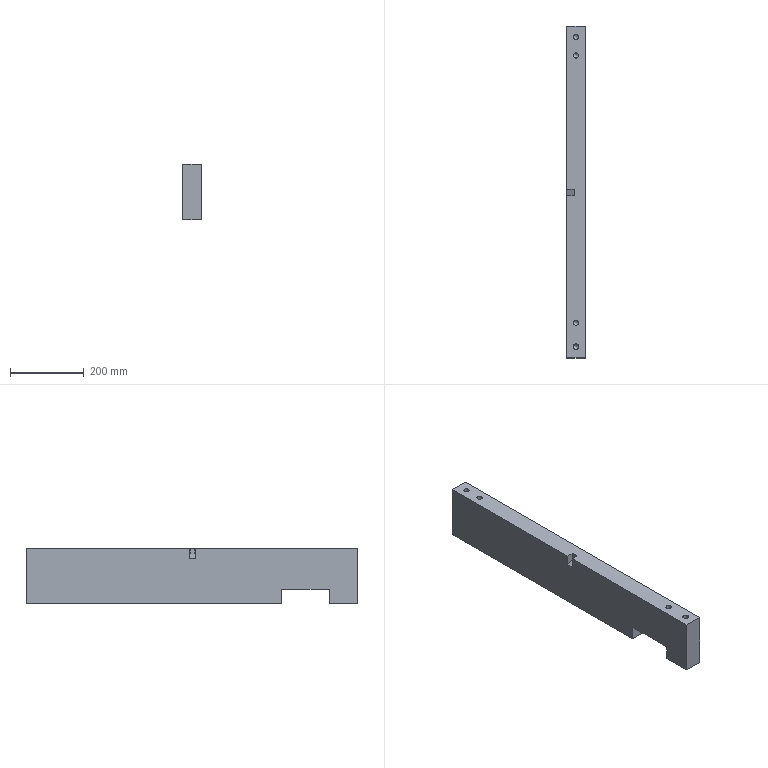Part | STEP file | 1_id1530_x_t | 1 solid | 29 faces | box 50 x 900 x 149.325 mm | volume 6417398 mm3 | plane 14 | cylinder 8 | cone 7 | commonest cylinder face diameters 14 x3 6 x2 10.716 x2 13.495 x1